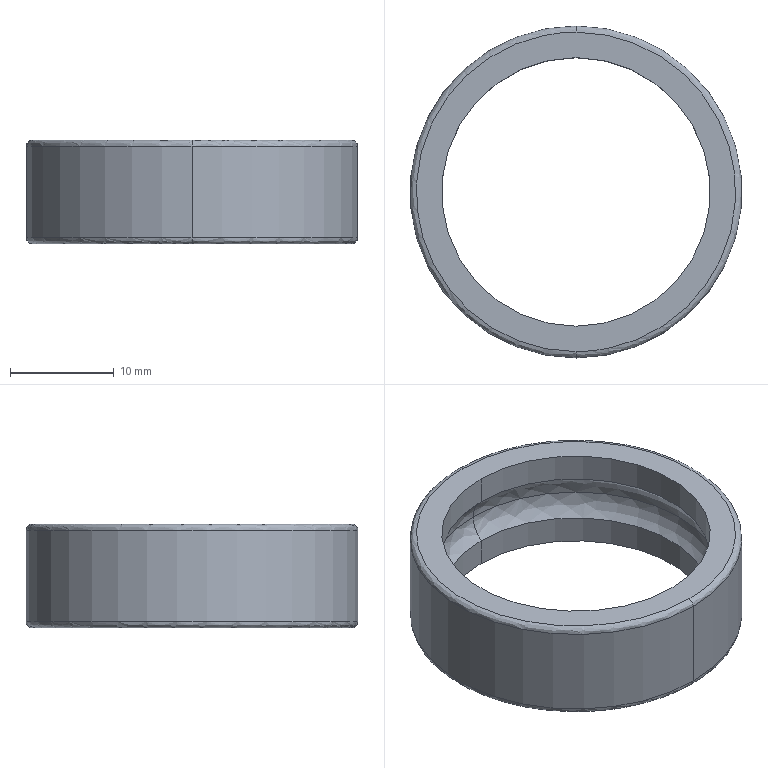Part | SolidWorks | features BaseBody 1 | 1 solid | 16 faces | box 32 x 32 x 10 mm | volume 2470 mm3 | spline 8 | cylinder 6 | plane 2 | commonest cylinder face diameters 25.9 x4 32 x2
STEP:
#1=CARTESIAN_POINT('',(0.,15.4,0.));
#2=VERTEX_POINT('',#1);
#3=CARTESIAN_POINT('',(0.,-15.4,0.));
#4=VERTEX_POINT('',#3);
#5=CARTESIAN_POINT('',(0.,15.4,0.));
#6=CARTESIAN_POINT('',(-30.8,15.4,0.));
#7=CARTESIAN_POINT('',(-30.8,-15.4,0.));
#8=CARTESIAN_POINT('',(0.,-15.4,0.));
#9=(BOUNDED_CURVE()B_SPLINE_CURVE(3,(#5,#6,#7,#8),.UNSPECIFIED.,.F.,.F.)B_SPLINE_CURVE_WITH_KNOTS((4,4),(0.25,0.75),.UNSPECIFIED.)CURVE()GEOMETRIC_REPRESENTATION_ITEM()RATIONAL_B_SPLINE_CURVE((1.,0.3333,0.3333,1.))REPRESENTATION_ITEM(''));
#10=EDGE_CURVE('',#2,#4,#9,.T.);
#11=ORIENTED_EDGE('',*,*,#10,.T.);
#12=CARTESIAN_POINT('',(0.,-16.,0.6));
#13=VERTEX_POINT('',#12);
#14=CARTESIAN_POINT('',(0.,-15.4,0.6));
#15=DIRECTION('',(-1.,0.,0.));
#16=DIRECTION('',(0.,-1.,0.));
#17=AXIS2_PLACEMENT_3D('',#14,#15,#16);
#18=CIRCLE('',#17,0.6);
#19=EDGE_CURVE('',#4,#13,#18,.T.);
#20=ORIENTED_EDGE('',*,*,#19,.T.);
#21=CARTESIAN_POINT('',(0.,16.,0.6));
#22=VERTEX_POINT('',#21);
#23=CARTESIAN_POINT('',(0.,0.,0.6));
#24=DIRECTION('',(0.,0.,1.));
#25=DIRECTION('',(0.,1.,0.));
#26=AXIS2_PLACEMENT_3D('',#23,#24,#25);
#27=CIRCLE('',#26,16.);
#28=EDGE_CURVE('',#22,#13,#27,.T.);
#29=ORIENTED_EDGE('',*,*,#28,.F.);
#30=CARTESIAN_POINT('',(0.,15.4,0.6));
#31=DIRECTION('',(1.,0.,0.));
#32=DIRECTION('',(0.,1.,0.));
#33=AXIS2_PLACEMENT_3D('',#30,#31,#32);
#34=CIRCLE('',#33,0.6);
#35=EDGE_CURVE('',#2,#22,#34,.T.);
#36=ORIENTED_EDGE('',*,*,#35,.F.);
#37=EDGE_LOOP('',(#11,#20,#29,#36));
#38=FACE_OUTER_BOUND('',#37,.T.);
#39=CARTESIAN_POINT('',(0.,-15.4,0.));
#40=CARTESIAN_POINT('',(-30.8,-15.4,0.));
#41=CARTESIAN_POINT('',(-30.8,15.4,0.));
#42=CARTESIAN_POINT('',(0.,15.4,0.));
#43=CARTESIAN_POINT('',(0.,-15.751,0.));
#44=CARTESIAN_POINT('',(-31.503,-15.751,0.));
#45=CARTESIAN_POINT('',(-31.503,15.751,0.));
#46=CARTESIAN_POINT('',(0.,15.751,0.));
#47=CARTESIAN_POINT('',(0.,-16.,0.2485));
#48=CARTESIAN_POINT('',(-32.,-16.,0.2485));
#49=CARTESIAN_POINT('',(-32.,16.,0.2485));
#50=CARTESIAN_POINT('',(0.,16.,0.2485));
#51=CARTESIAN_POINT('',(0.,-16.,0.6));
#52=CARTESIAN_POINT('',(-32.,-16.,0.6));
#53=CARTESIAN_POINT('',(-32.,16.,0.6));
#54=CARTESIAN_POINT('',(0.,16.,0.6));
#55=(BOUNDED_SURFACE()B_SPLINE_SURFACE(3,3,((#39,#40,#41,#42),(#43,#44,#45,#46),(#47,#48,#49,#50),(#51,#52,#53,#54)),.UNSPECIFIED.,.F.,.F.,.T.)B_SPLINE_SURFACE_WITH_KNOTS((4,4),(4,4),(0.,1.),(0.,1.),.UNSPECIFIED.)GEOMETRIC_REPRESENTATION_ITEM()RATIONAL_B_SPLINE_SURFACE(((1.,0.3333,0.3333,1.),(0.8047,0.2682,0.2682,0.8047),(0.8047,0.2682,0.2682,0.8047),(1.,0.3333,0.3333,1.)))REPRESENTATION_ITEM('')SURFACE());
#56=ADVANCED_FACE('',(#38),#55,.T.);
#57=CARTESIAN_POINT('',(0.,-16.,9.4));
#58=VERTEX_POINT('',#57);
#59=CARTESIAN_POINT('',(0.,16.,9.4));
#60=VERTEX_POINT('',#59);
#61=CARTESIAN_POINT('',(0.,0.,9.4));
#62=DIRECTION('',(0.,0.,-1.));
#63=DIRECTION('',(0.,1.,0.));
#64=AXIS2_PLACEMENT_3D('',#61,#62,#63);
#65=CIRCLE('',#64,16.);
#66=EDGE_CURVE('',#58,#60,#65,.T.);
#67=ORIENTED_EDGE('',*,*,#66,.F.);
#68=CARTESIAN_POINT('',(0.,-15.4,10.));
#69=VERTEX_POINT('',#68);
#70=CARTESIAN_POINT('',(0.,-15.4,9.4));
#71=DIRECTION('',(-1.,0.,0.));
#72=DIRECTION('',(0.,-1.,0.));
#73=AXIS2_PLACEMENT_3D('',#70,#71,#72);
#74=CIRCLE('',#73,0.6);
#75=EDGE_CURVE('',#58,#69,#74,.T.);
#76=ORIENTED_EDGE('',*,*,#75,.T.);
#77=CARTESIAN_POINT('',(0.,15.4,10.));
#78=VERTEX_POINT('',#77);
#79=CARTESIAN_POINT('',(0.,-15.4,10.));
#80=CARTESIAN_POINT('',(-30.8,-15.4,10.));
#81=CARTESIAN_POINT('',(-30.8,15.4,10.));
#82=CARTESIAN_POINT('',(0.,15.4,10.));
#83=(BOUNDED_CURVE()B_SPLINE_CURVE(3,(#79,#80,#81,#82),.UNSPECIFIED.,.F.,.F.)B_SPLINE_CURVE_WITH_KNOTS((4,4),(0.25,0.75),.UNSPECIFIED.)CURVE()GEOMETRIC_REPRESENTATION_ITEM()RATIONAL_B_SPLINE_CURVE((1.,0.3333,0.3333,1.))REPRESENTATION_ITEM(''));
#84=EDGE_CURVE('',#69,#78,#83,.T.);
#85=ORIENTED_EDGE('',*,*,#84,.T.);
#86=CARTESIAN_POINT('',(0.,15.4,9.4));
#87=DIRECTION('',(1.,0.,0.));
#88=DIRECTION('',(0.,1.,0.));
#89=AXIS2_PLACEMENT_3D('',#86,#87,#88);
#90=CIRCLE('',#89,0.6);
#91=EDGE_CURVE('',#60,#78,#90,.T.);
#92=ORIENTED_EDGE('',*,*,#91,.F.);
#93=EDGE_LOOP('',(#67,#76,#85,#92));
#94=FACE_OUTER_BOUND('',#93,.T.);
#95=CARTESIAN_POINT('',(0.,-16.,9.4));
#96=CARTESIAN_POINT('',(-32.,-16.,9.4));
#97=CARTESIAN_POINT('',(-32.,16.,9.4));
#98=CARTESIAN_POINT('',(0.,16.,9.4));
#99=CARTESIAN_POINT('',(0.,-16.,9.751));
#100=CARTESIAN_POINT('',(-32.,-16.,9.751));
#101=CARTESIAN_POINT('',(-32.,16.,9.751));
#102=CARTESIAN_POINT('',(0.,16.,9.751));
#103=CARTESIAN_POINT('',(0.,-15.751,10.));
#104=CARTESIAN_POINT('',(-31.503,-15.751,10.));
#105=CARTESIAN_POINT('',(-31.503,15.751,10.));
#106=CARTESIAN_POINT('',(0.,15.751,10.));
#107=CARTESIAN_POINT('',(0.,-15.4,10.));
#108=CARTESIAN_POINT('',(-30.8,-15.4,10.));
#109=CARTESIAN_POINT('',(-30.8,15.4,10.));
#110=CARTESIAN_POINT('',(0.,15.4,10.));
#111=(BOUNDED_SURFACE()B_SPLINE_SURFACE(3,3,((#95,#96,#97,#98),(#99,#100,#101,#102),(#103,#104,#105,#106),(#107,#108,#109,#110)),.UNSPECIFIED.,.F.,.F.,.T.)B_SPLINE_SURFACE_WITH_KNOTS((4,4),(4,4),(0.,1.),(0.,1.),.UNSPECIFIED.)GEOMETRIC_REPRESENTATION_ITEM()RATIONAL_B_SPLINE_SURFACE(((1.,0.3333,0.3333,1.),(0.8047,0.2682,0.2682,0.8047),(0.8047,0.2682,0.2682,0.8047),(1.,0.3333,0.3333,1.)))REPRESENTATION_ITEM('')SURFACE());
#112=ADVANCED_FACE('',(#94),#111,.T.);
#113=CARTESIAN_POINT('',(0.,12.95,2.699));
#114=VERTEX_POINT('',#113);
#115=CARTESIAN_POINT('',(0.,-12.95,2.699));
#116=VERTEX_POINT('',#115);
#117=CARTESIAN_POINT('',(0.,0.,2.699));
#118=DIRECTION('',(0.,0.,-1.));
#119=DIRECTION('',(0.,1.,0.));
#120=AXIS2_PLACEMENT_3D('',#117,#118,#119);
#121=CIRCLE('',#120,12.95);
#122=EDGE_CURVE('',#114,#116,#121,.T.);
#123=ORIENTED_EDGE('',*,*,#122,.T.);
#124=CARTESIAN_POINT('',(0.,-14.025,5.));
#125=VERTEX_POINT('',#124);
#126=CARTESIAN_POINT('',(0.,-11.025,5.));
#127=DIRECTION('',(-1.,0.,0.));
#128=DIRECTION('',(0.,-1.,0.));
#129=AXIS2_PLACEMENT_3D('',#126,#127,#128);
#130=CIRCLE('',#129,3.);
#131=EDGE_CURVE('',#116,#125,#130,.T.);
#132=ORIENTED_EDGE('',*,*,#131,.T.);
#133=CARTESIAN_POINT('',(0.,14.025,5.));
#134=VERTEX_POINT('',#133);
#135=CARTESIAN_POINT('',(0.,0.,5.));
#136=DIRECTION('',(0.,0.,-1.));
#137=DIRECTION('',(0.,1.,0.));
#138=AXIS2_PLACEMENT_3D('',#135,#136,#137);
#139=CIRCLE('',#138,14.025);
#140=EDGE_CURVE('',#134,#125,#139,.T.);
#141=ORIENTED_EDGE('',*,*,#140,.F.);
#142=CARTESIAN_POINT('',(0.,11.025,5.));
#143=DIRECTION('',(1.,0.,0.));
#144=DIRECTION('',(0.,1.,0.));
#145=AXIS2_PLACEMENT_3D('',#142,#143,#144);
#146=CIRCLE('',#145,3.);
#147=EDGE_CURVE('',#114,#134,#146,.T.);
#148=ORIENTED_EDGE('',*,*,#147,.F.);
#149=EDGE_LOOP('',(#123,#132,#141,#148));
#150=FACE_OUTER_BOUND('',#149,.T.);
#151=CARTESIAN_POINT('',(0.,12.95,2.699));
#152=CARTESIAN_POINT('',(25.9,12.95,2.699));
#153=CARTESIAN_POINT('',(25.9,-12.95,2.699));
#154=CARTESIAN_POINT('',(0.,-12.95,2.699));
#155=CARTESIAN_POINT('',(0.,13.643,3.279));
#156=CARTESIAN_POINT('',(27.285,13.643,3.279));
#157=CARTESIAN_POINT('',(27.285,-13.643,3.279));
#158=CARTESIAN_POINT('',(0.,-13.643,3.279));
#159=CARTESIAN_POINT('',(0.,14.025,4.097));
#160=CARTESIAN_POINT('',(28.05,14.025,4.097));
#161=CARTESIAN_POINT('',(28.05,-14.025,4.097));
#162=CARTESIAN_POINT('',(0.,-14.025,4.097));
#163=CARTESIAN_POINT('',(0.,14.025,5.));
#164=CARTESIAN_POINT('',(28.05,14.025,5.));
#165=CARTESIAN_POINT('',(28.05,-14.025,5.));
#166=CARTESIAN_POINT('',(0.,-14.025,5.));
#167=(BOUNDED_SURFACE()B_SPLINE_SURFACE(3,3,((#151,#152,#153,#154),(#155,#156,#157,#158),(#159,#160,#161,#162),(#163,#164,#165,#166)),.UNSPECIFIED.,.F.,.F.,.T.)B_SPLINE_SURFACE_WITH_KNOTS((4,4),(4,4),(0.,1.),(0.,1.),.UNSPECIFIED.)GEOMETRIC_REPRESENTATION_ITEM()RATIONAL_B_SPLINE_SURFACE(((1.,0.3333,0.3333,1.),(0.9373,0.3124,0.3124,0.9373),(0.9373,0.3124,0.3124,0.9373),(1.,0.3333,0.3333,1.)))REPRESENTATION_ITEM('')SURFACE());
#168=ADVANCED_FACE('',(#150),#167,.F.);
#169=ORIENTED_EDGE('',*,*,#140,.T.);
#170=CARTESIAN_POINT('',(0.,-12.95,7.301));
#171=VERTEX_POINT('',#170);
#172=CARTESIAN_POINT('',(0.,-11.025,5.));
#173=DIRECTION('',(-1.,0.,0.));
#174=DIRECTION('',(0.,-1.,0.));
#175=AXIS2_PLACEMENT_3D('',#172,#173,#174);
#176=CIRCLE('',#175,3.);
#177=EDGE_CURVE('',#125,#171,#176,.T.);
#178=ORIENTED_EDGE('',*,*,#177,.T.);
#179=CARTESIAN_POINT('',(0.,12.95,7.301));
#180=VERTEX_POINT('',#179);
#181=CARTESIAN_POINT('',(0.,0.,7.301));
#182=DIRECTION('',(0.,0.,1.));
#183=DIRECTION('',(0.,1.,0.));
#184=AXIS2_PLACEMENT_3D('',#181,#182,#183);
#185=CIRCLE('',#184,12.95);
#186=EDGE_CURVE('',#171,#180,#185,.T.);
#187=ORIENTED_EDGE('',*,*,#186,.T.);
#188=CARTESIAN_POINT('',(0.,11.025,5.));
#189=DIRECTION('',(1.,0.,0.));
#190=DIRECTION('',(0.,1.,0.));
#191=AXIS2_PLACEMENT_3D('',#188,#189,#190);
#192=CIRCLE('',#191,3.);
#193=EDGE_CURVE('',#134,#180,#192,.T.);
#194=ORIENTED_EDGE('',*,*,#193,.F.);
#195=EDGE_LOOP('',(#169,#178,#187,#194));
#196=FACE_OUTER_BOUND('',#195,.T.);
#197=CARTESIAN_POINT('',(0.,14.025,5.));
#198=CARTESIAN_POINT('',(28.05,14.025,5.));
#199=CARTESIAN_POINT('',(28.05,-14.025,5.));
#200=CARTESIAN_POINT('',(0.,-14.025,5.));
#201=CARTESIAN_POINT('',(0.,14.025,5.903));
#202=CARTESIAN_POINT('',(28.05,14.025,5.903));
#203=CARTESIAN_POINT('',(28.05,-14.025,5.903));
#204=CARTESIAN_POINT('',(0.,-14.025,5.903));
#205=CARTESIAN_POINT('',(0.,13.643,6.721));
#206=CARTESIAN_POINT('',(27.285,13.643,6.721));
#207=CARTESIAN_POINT('',(27.285,-13.643,6.721));
#208=CARTESIAN_POINT('',(0.,-13.643,6.721));
#209=CARTESIAN_POINT('',(0.,12.95,7.301));
#210=CARTESIAN_POINT('',(25.9,12.95,7.301));
#211=CARTESIAN_POINT('',(25.9,-12.95,7.301));
#212=CARTESIAN_POINT('',(0.,-12.95,7.301));
#213=(BOUNDED_SURFACE()B_SPLINE_SURFACE(3,3,((#197,#198,#199,#200),(#201,#202,#203,#204),(#205,#206,#207,#208),(#209,#210,#211,#212)),.UNSPECIFIED.,.F.,.F.,.F.)B_SPLINE_SURFACE_WITH_KNOTS((4,4),(4,4),(0.,1.),(0.,1.),.UNSPECIFIED.)GEOMETRIC_REPRESENTATION_ITEM()RATIONAL_B_SPLINE_SURFACE(((1.,0.3333,0.3333,1.),(0.9373,0.3124,0.3124,0.9373),(0.9373,0.3124,0.3124,0.9373),(1.,0.3333,0.3333,1.)))REPRESENTATION_ITEM('')SURFACE());
#214=ADVANCED_FACE('',(#196),#213,.F.);
#215=CARTESIAN_POINT('',(0.,0.,9.4));
#216=DIRECTION('',(0.,0.,-1.));
#217=DIRECTION('',(0.,1.,0.));
#218=AXIS2_PLACEMENT_3D('',#215,#216,#217);
#219=CIRCLE('',#218,16.);
#220=EDGE_CURVE('',#60,#58,#219,.T.);
#221=ORIENTED_EDGE('',*,*,#220,.T.);
#222=CARTESIAN_POINT('',(0.,-16.,0.));
#223=DIRECTION('',(0.,0.,-1.));
#224=VECTOR('',#223,1000.);
#225=LINE('',#222,#224);
#226=EDGE_CURVE('',#58,#13,#225,.T.);
#227=ORIENTED_EDGE('',*,*,#226,.T.);
#228=CARTESIAN_POINT('',(0.,0.,0.6));
#229=DIRECTION('',(0.,0.,1.));
#230=DIRECTION('',(0.,1.,0.));
#231=AXIS2_PLACEMENT_3D('',#228,#229,#230);
#232=CIRCLE('',#231,16.);
#233=EDGE_CURVE('',#13,#22,#232,.T.);
#234=ORIENTED_EDGE('',*,*,#233,.T.);
#235=CARTESIAN_POINT('',(0.,16.,0.));
#236=DIRECTION('',(0.,0.,-1.));
#237=VECTOR('',#236,1000.);
#238=LINE('',#235,#237);
#239=EDGE_CURVE('',#60,#22,#238,.T.);
#240=ORIENTED_EDGE('',*,*,#239,.F.);
#241=EDGE_LOOP('',(#221,#227,#234,#240));
#242=FACE_OUTER_BOUND('',#241,.T.);
#243=CARTESIAN_POINT('',(0.,0.,0.));
#244=DIRECTION('',(0.,0.,-1.));
#245=DIRECTION('',(0.,1.,0.));
#246=AXIS2_PLACEMENT_3D('',#243,#244,#245);
#247=CYLINDRICAL_SURFACE('',#246,16.);
#248=ADVANCED_FACE('',(#242),#247,.T.);
#249=CARTESIAN_POINT('',(0.,0.,2.699));
#250=DIRECTION('',(0.,0.,-1.));
#251=DIRECTION('',(0.,1.,0.));
#252=AXIS2_PLACEMENT_3D('',#249,#250,#251);
#253=CIRCLE('',#252,12.95);
#254=EDGE_CURVE('',#116,#114,#253,.T.);
#255=ORIENTED_EDGE('',*,*,#254,.F.);
#256=CARTESIAN_POINT('',(0.,-12.95,0.));
#257=VERTEX_POINT('',#256);
#258=CARTESIAN_POINT('',(0.,-12.95,0.));
#259=DIRECTION('',(0.,0.,-1.));
#260=VECTOR('',#259,1000.);
#261=LINE('',#258,#260);
#262=EDGE_CURVE('',#116,#257,#261,.T.);
#263=ORIENTED_EDGE('',*,*,#262,.T.);
#264=CARTESIAN_POINT('',(0.,12.95,0.));
#265=VERTEX_POINT('',#264);
#266=CARTESIAN_POINT('',(0.,0.,0.));
#267=DIRECTION('',(0.,0.,1.));
#268=DIRECTION('',(0.,1.,0.));
#269=AXIS2_PLACEMENT_3D('',#266,#267,#268);
#270=CIRCLE('',#269,12.95);
#271=EDGE_CURVE('',#265,#257,#270,.T.);
#272=ORIENTED_EDGE('',*,*,#271,.F.);
#273=CARTESIAN_POINT('',(0.,12.95,0.));
#274=DIRECTION('',(0.,0.,-1.));
#275=VECTOR('',#274,1000.);
#276=LINE('',#273,#275);
#277=EDGE_CURVE('',#114,#265,#276,.T.);
#278=ORIENTED_EDGE('',*,*,#277,.F.);
#279=EDGE_LOOP('',(#255,#263,#272,#278));
#280=FACE_OUTER_BOUND('',#279,.T.);
#281=CARTESIAN_POINT('',(0.,0.,0.));
#282=DIRECTION('',(0.,0.,-1.));
#283=DIRECTION('',(0.,1.,0.));
#284=AXIS2_PLACEMENT_3D('',#281,#282,#283);
#285=CYLINDRICAL_SURFACE('',#284,12.95);
#286=ADVANCED_FACE('',(#280),#285,.F.);
#287=CARTESIAN_POINT('',(0.,-12.95,10.));
#288=VERTEX_POINT('',#287);
#289=CARTESIAN_POINT('',(0.,12.95,10.));
#290=VERTEX_POINT('',#289);
#291=CARTESIAN_POINT('',(0.,0.,10.));
#292=DIRECTION('',(0.,0.,-1.));
#293=DIRECTION('',(0.,1.,0.));
#294=AXIS2_PLACEMENT_3D('',#291,#292,#293);
#295=CIRCLE('',#294,12.95);
#296=EDGE_CURVE('',#288,#290,#295,.T.);
#297=ORIENTED_EDGE('',*,*,#296,.F.);
#298=CARTESIAN_POINT('',(0.,-12.95,0.));
#299=DIRECTION('',(0.,0.,-1.));
#300=VECTOR('',#299,1000.);
#301=LINE('',#298,#300);
#302=EDGE_CURVE('',#288,#171,#301,.T.);
#303=ORIENTED_EDGE('',*,*,#302,.T.);
#304=CARTESIAN_POINT('',(0.,0.,7.301));
#305=DIRECTION('',(0.,0.,1.));
#306=DIRECTION('',(0.,1.,0.));
#307=AXIS2_PLACEMENT_3D('',#304,#305,#306);
#308=CIRCLE('',#307,12.95);
#309=EDGE_CURVE('',#180,#171,#308,.T.);
#310=ORIENTED_EDGE('',*,*,#309,.F.);
#311=CARTESIAN_POINT('',(0.,12.95,0.));
#312=DIRECTION('',(0.,0.,-1.));
#313=VECTOR('',#312,1000.);
#314=LINE('',#311,#313);
#315=EDGE_CURVE('',#290,#180,#314,.T.);
#316=ORIENTED_EDGE('',*,*,#315,.F.);
#317=EDGE_LOOP('',(#297,#303,#310,#316));
#318=FACE_OUTER_BOUND('',#317,.T.);
#319=CARTESIAN_POINT('',(0.,0.,0.));
#320=DIRECTION('',(0.,0.,-1.));
#321=DIRECTION('',(0.,1.,0.));
#322=AXIS2_PLACEMENT_3D('',#319,#320,#321);
#323=CYLINDRICAL_SURFACE('',#322,12.95);
#324=ADVANCED_FACE('',(#318),#323,.F.);
#325=ORIENTED_EDGE('',*,*,#177,.F.);
#326=CARTESIAN_POINT('',(0.,0.,5.));
#327=DIRECTION('',(0.,0.,-1.));
#328=DIRECTION('',(0.,1.,0.));
#329=AXIS2_PLACEMENT_3D('',#326,#327,#328);
#330=CIRCLE('',#329,14.025);
#331=EDGE_CURVE('',#125,#134,#330,.T.);
#332=ORIENTED_EDGE('',*,*,#331,.T.);
#333=ORIENTED_EDGE('',*,*,#193,.T.);
#334=ORIENTED_EDGE('',*,*,#309,.T.);
#335=EDGE_LOOP('',(#325,#332,#333,#334));
#336=FACE_OUTER_BOUND('',#335,.T.);
#337=CARTESIAN_POINT('',(0.,-14.025,5.));
#338=CARTESIAN_POINT('',(-28.05,-14.025,5.));
#339=CARTESIAN_POINT('',(-28.05,14.025,5.));
#340=CARTESIAN_POINT('',(0.,14.025,5.));
#341=CARTESIAN_POINT('',(0.,-14.025,5.903));
#342=CARTESIAN_POINT('',(-28.05,-14.025,5.903));
#343=CARTESIAN_POINT('',(-28.05,14.025,5.903));
#344=CARTESIAN_POINT('',(0.,14.025,5.903));
#345=CARTESIAN_POINT('',(0.,-13.643,6.721));
#346=CARTESIAN_POINT('',(-27.285,-13.643,6.721));
#347=CARTESIAN_POINT('',(-27.285,13.643,6.721));
#348=CARTESIAN_POINT('',(0.,13.643,6.721));
#349=CARTESIAN_POINT('',(0.,-12.95,7.301));
#350=CARTESIAN_POINT('',(-25.9,-12.95,7.301));
#351=CARTESIAN_POINT('',(-25.9,12.95,7.301));
#352=CARTESIAN_POINT('',(0.,12.95,7.301));
#353=(BOUNDED_SURFACE()B_SPLINE_SURFACE(3,3,((#337,#338,#339,#340),(#341,#342,#343,#344),(#345,#346,#347,#348),(#349,#350,#351,#352)),.UNSPECIFIED.,.F.,.F.,.T.)B_SPLINE_SURFACE_WITH_KNOTS((4,4),(4,4),(0.,1.),(0.,1.),.UNSPECIFIED.)GEOMETRIC_REPRESENTATION_ITEM()RATIONAL_B_SPLINE_SURFACE(((1.,0.3333,0.3333,1.),(0.9373,0.3124,0.3124,0.9373),(0.9373,0.3124,0.3124,0.9373),(1.,0.3333,0.3333,1.)))REPRESENTATION_ITEM('')SURFACE());
#354=ADVANCED_FACE('',(#336),#353,.F.);
#355=ORIENTED_EDGE('',*,*,#226,.F.);
#356=ORIENTED_EDGE('',*,*,#66,.T.);
#357=ORIENTED_EDGE('',*,*,#239,.T.);
#358=ORIENTED_EDGE('',*,*,#28,.T.);
#359=EDGE_LOOP('',(#355,#356,#357,#358));
#360=FACE_OUTER_BOUND('',#359,.T.);
#361=CARTESIAN_POINT('',(0.,0.,0.));
#362=DIRECTION('',(0.,0.,-1.));
#363=DIRECTION('',(0.,1.,0.));
#364=AXIS2_PLACEMENT_3D('',#361,#362,#363);
#365=CYLINDRICAL_SURFACE('',#364,16.);
#366=ADVANCED_FACE('',(#360),#365,.T.);
#367=ORIENTED_EDGE('',*,*,#19,.F.);
#368=CARTESIAN_POINT('',(0.,-15.4,0.));
#369=CARTESIAN_POINT('',(30.8,-15.4,0.));
#370=CARTESIAN_POINT('',(30.8,15.4,0.));
#371=CARTESIAN_POINT('',(0.,15.4,0.));
#372=(BOUNDED_CURVE()B_SPLINE_CURVE(3,(#368,#369,#370,#371),.UNSPECIFIED.,.F.,.F.)B_SPLINE_CURVE_WITH_KNOTS((4,4),(0.75,1.25),.UNSPECIFIED.)CURVE()GEOMETRIC_REPRESENTATION_ITEM()RATIONAL_B_SPLINE_CURVE((1.,0.3333,0.3333,1.))REPRESENTATION_ITEM(''));
#373=EDGE_CURVE('',#4,#2,#372,.T.);
#374=ORIENTED_EDGE('',*,*,#373,.T.);
#375=ORIENTED_EDGE('',*,*,#35,.T.);
#376=ORIENTED_EDGE('',*,*,#233,.F.);
#377=EDGE_LOOP('',(#367,#374,#375,#376));
#378=FACE_OUTER_BOUND('',#377,.T.);
#379=CARTESIAN_POINT('',(0.,15.4,0.));
#380=CARTESIAN_POINT('',(30.8,15.4,0.));
#381=CARTESIAN_POINT('',(30.8,-15.4,0.));
#382=CARTESIAN_POINT('',(0.,-15.4,0.));
#383=CARTESIAN_POINT('',(0.,15.751,0.));
#384=CARTESIAN_POINT('',(31.503,15.751,0.));
#385=CARTESIAN_POINT('',(31.503,-15.751,0.));
#386=CARTESIAN_POINT('',(0.,-15.751,0.));
#387=CARTESIAN_POINT('',(0.,16.,0.2485));
#388=CARTESIAN_POINT('',(32.,16.,0.2485));
#389=CARTESIAN_POINT('',(32.,-16.,0.2485));
#390=CARTESIAN_POINT('',(0.,-16.,0.2485));
#391=CARTESIAN_POINT('',(0.,16.,0.6));
#392=CARTESIAN_POINT('',(32.,16.,0.6));
#393=CARTESIAN_POINT('',(32.,-16.,0.6));
#394=CARTESIAN_POINT('',(0.,-16.,0.6));
#395=(BOUNDED_SURFACE()B_SPLINE_SURFACE(3,3,((#379,#380,#381,#382),(#383,#384,#385,#386),(#387,#388,#389,#390),(#391,#392,#393,#394)),.UNSPECIFIED.,.F.,.F.,.T.)B_SPLINE_SURFACE_WITH_KNOTS((4,4),(4,4),(0.,1.),(0.,1.),.UNSPECIFIED.)GEOMETRIC_REPRESENTATION_ITEM()RATIONAL_B_SPLINE_SURFACE(((1.,0.3333,0.3333,1.),(0.8047,0.2682,0.2682,0.8047),(0.8047,0.2682,0.2682,0.8047),(1.,0.3333,0.3333,1.)))REPRESENTATION_ITEM('')SURFACE());
#396=ADVANCED_FACE('',(#378),#395,.T.);
#397=ORIENTED_EDGE('',*,*,#75,.F.);
#398=ORIENTED_EDGE('',*,*,#220,.F.);
#399=ORIENTED_EDGE('',*,*,#91,.T.);
#400=CARTESIAN_POINT('',(0.,15.4,10.));
#401=CARTESIAN_POINT('',(30.8,15.4,10.));
#402=CARTESIAN_POINT('',(30.8,-15.4,10.));
#403=CARTESIAN_POINT('',(0.,-15.4,10.));
#404=(BOUNDED_CURVE()B_SPLINE_CURVE(3,(#400,#401,#402,#403),.UNSPECIFIED.,.F.,.F.)B_SPLINE_CURVE_WITH_KNOTS((4,4),(0.75,1.25),.UNSPECIFIED.)CURVE()GEOMETRIC_REPRESENTATION_ITEM()RATIONAL_B_SPLINE_CURVE((1.,0.3333,0.3333,1.))REPRESENTATION_ITEM(''));
#405=EDGE_CURVE('',#78,#69,#404,.T.);
#406=ORIENTED_EDGE('',*,*,#405,.T.);
#407=EDGE_LOOP('',(#397,#398,#399,#406));
#408=FACE_OUTER_BOUND('',#407,.T.);
#409=CARTESIAN_POINT('',(0.,16.,9.4));
#410=CARTESIAN_POINT('',(32.,16.,9.4));
#411=CARTESIAN_POINT('',(32.,-16.,9.4));
#412=CARTESIAN_POINT('',(0.,-16.,9.4));
#413=CARTESIAN_POINT('',(0.,16.,9.751));
#414=CARTESIAN_POINT('',(32.,16.,9.751));
#415=CARTESIAN_POINT('',(32.,-16.,9.751));
#416=CARTESIAN_POINT('',(0.,-16.,9.751));
#417=CARTESIAN_POINT('',(0.,15.751,10.));
#418=CARTESIAN_POINT('',(31.503,15.751,10.));
#419=CARTESIAN_POINT('',(31.503,-15.751,10.));
#420=CARTESIAN_POINT('',(0.,-15.751,10.));
#421=CARTESIAN_POINT('',(0.,15.4,10.));
#422=CARTESIAN_POINT('',(30.8,15.4,10.));
#423=CARTESIAN_POINT('',(30.8,-15.4,10.));
#424=CARTESIAN_POINT('',(0.,-15.4,10.));
#425=(BOUNDED_SURFACE()B_SPLINE_SURFACE(3,3,((#409,#410,#411,#412),(#413,#414,#415,#416),(#417,#418,#419,#420),(#421,#422,#423,#424)),.UNSPECIFIED.,.F.,.F.,.T.)B_SPLINE_SURFACE_WITH_KNOTS((4,4),(4,4),(0.,1.),(0.,1.),.UNSPECIFIED.)GEOMETRIC_REPRESENTATION_ITEM()RATIONAL_B_SPLINE_SURFACE(((1.,0.3333,0.3333,1.),(0.8047,0.2682,0.2682,0.8047),(0.8047,0.2682,0.2682,0.8047),(1.,0.3333,0.3333,1.)))REPRESENTATION_ITEM('')SURFACE());
#426=ADVANCED_FACE('',(#408),#425,.T.);
#427=ORIENTED_EDGE('',*,*,#271,.T.);
#428=CARTESIAN_POINT('',(0.,0.,0.));
#429=DIRECTION('',(0.,0.,1.));
#430=DIRECTION('',(0.,1.,0.));
#431=AXIS2_PLACEMENT_3D('',#428,#429,#430);
#432=CIRCLE('',#431,12.95);
#433=EDGE_CURVE('',#257,#265,#432,.T.);
#434=ORIENTED_EDGE('',*,*,#433,.T.);
#435=EDGE_LOOP('',(#427,#434));
#436=FACE_BOUND('',#435,.T.);
#437=ORIENTED_EDGE('',*,*,#10,.F.);
#438=ORIENTED_EDGE('',*,*,#373,.F.);
#439=EDGE_LOOP('',(#437,#438));
#440=FACE_OUTER_BOUND('',#439,.T.);
#441=CARTESIAN_POINT('',(12.95,0.,0.));
#442=DIRECTION('',(0.,0.,-1.));
#443=DIRECTION('',(0.,1.,0.));
#444=AXIS2_PLACEMENT_3D('',#441,#442,#443);
#445=PLANE('',#444);
#446=ADVANCED_FACE('',(#436,#440),#445,.T.);
#447=ORIENTED_EDGE('',*,*,#405,.F.);
#448=ORIENTED_EDGE('',*,*,#84,.F.);
#449=EDGE_LOOP('',(#447,#448));
#450=FACE_OUTER_BOUND('',#449,.T.);
#451=CARTESIAN_POINT('',(0.,0.,10.));
#452=DIRECTION('',(0.,0.,-1.));
#453=DIRECTION('',(0.,1.,0.));
#454=AXIS2_PLACEMENT_3D('',#451,#452,#453);
#455=CIRCLE('',#454,12.95);
#456=EDGE_CURVE('',#290,#288,#455,.T.);
#457=ORIENTED_EDGE('',*,*,#456,.T.);
#458=ORIENTED_EDGE('',*,*,#296,.T.);
#459=EDGE_LOOP('',(#457,#458));
#460=FACE_BOUND('',#459,.T.);
#461=CARTESIAN_POINT('',(15.4,0.,10.));
#462=DIRECTION('',(0.,0.,1.));
#463=DIRECTION('',(0.,-1.,0.));
#464=AXIS2_PLACEMENT_3D('',#461,#462,#463);
#465=PLANE('',#464);
#466=ADVANCED_FACE('',(#450,#460),#465,.T.);
#467=ORIENTED_EDGE('',*,*,#262,.F.);
#468=ORIENTED_EDGE('',*,*,#122,.F.);
#469=ORIENTED_EDGE('',*,*,#277,.T.);
#470=ORIENTED_EDGE('',*,*,#433,.F.);
#471=EDGE_LOOP('',(#467,#468,#469,#470));
#472=FACE_OUTER_BOUND('',#471,.T.);
#473=CARTESIAN_POINT('',(0.,0.,0.));
#474=DIRECTION('',(0.,0.,-1.));
#475=DIRECTION('',(0.,1.,0.));
#476=AXIS2_PLACEMENT_3D('',#473,#474,#475);
#477=CYLINDRICAL_SURFACE('',#476,12.95);
#478=ADVANCED_FACE('',(#472),#477,.F.);
#479=ORIENTED_EDGE('',*,*,#302,.F.);
#480=ORIENTED_EDGE('',*,*,#456,.F.);
#481=ORIENTED_EDGE('',*,*,#315,.T.);
#482=ORIENTED_EDGE('',*,*,#186,.F.);
#483=EDGE_LOOP('',(#479,#480,#481,#482));
#484=FACE_OUTER_BOUND('',#483,.T.);
#485=CARTESIAN_POINT('',(0.,0.,0.));
#486=DIRECTION('',(0.,0.,-1.));
#487=DIRECTION('',(0.,1.,0.));
#488=AXIS2_PLACEMENT_3D('',#485,#486,#487);
#489=CYLINDRICAL_SURFACE('',#488,12.95);
#490=ADVANCED_FACE('',(#484),#489,.F.);
#491=ORIENTED_EDGE('',*,*,#131,.F.);
#492=ORIENTED_EDGE('',*,*,#254,.T.);
#493=ORIENTED_EDGE('',*,*,#147,.T.);
#494=ORIENTED_EDGE('',*,*,#331,.F.);
#495=EDGE_LOOP('',(#491,#492,#493,#494));
#496=FACE_OUTER_BOUND('',#495,.T.);
#497=CARTESIAN_POINT('',(0.,-12.95,2.699));
#498=CARTESIAN_POINT('',(-25.9,-12.95,2.699));
#499=CARTESIAN_POINT('',(-25.9,12.95,2.699));
#500=CARTESIAN_POINT('',(0.,12.95,2.699));
#501=CARTESIAN_POINT('',(0.,-13.643,3.279));
#502=CARTESIAN_POINT('',(-27.285,-13.643,3.279));
#503=CARTESIAN_POINT('',(-27.285,13.643,3.279));
#504=CARTESIAN_POINT('',(0.,13.643,3.279));
#505=CARTESIAN_POINT('',(0.,-14.025,4.097));
#506=CARTESIAN_POINT('',(-28.05,-14.025,4.097));
#507=CARTESIAN_POINT('',(-28.05,14.025,4.097));
#508=CARTESIAN_POINT('',(0.,14.025,4.097));
#509=CARTESIAN_POINT('',(0.,-14.025,5.));
#510=CARTESIAN_POINT('',(-28.05,-14.025,5.));
#511=CARTESIAN_POINT('',(-28.05,14.025,5.));
#512=CARTESIAN_POINT('',(0.,14.025,5.));
#513=(BOUNDED_SURFACE()B_SPLINE_SURFACE(3,3,((#497,#498,#499,#500),(#501,#502,#503,#504),(#505,#506,#507,#508),(#509,#510,#511,#512)),.UNSPECIFIED.,.F.,.F.,.F.)B_SPLINE_SURFACE_WITH_KNOTS((4,4),(4,4),(0.,1.),(0.,1.),.UNSPECIFIED.)GEOMETRIC_REPRESENTATION_ITEM()RATIONAL_B_SPLINE_SURFACE(((1.,0.3333,0.3333,1.),(0.9373,0.3124,0.3124,0.9373),(0.9373,0.3124,0.3124,0.9373),(1.,0.3333,0.3333,1.)))REPRESENTATION_ITEM('')SURFACE());
#514=ADVANCED_FACE('',(#496),#513,.F.);
#515=CLOSED_SHELL('',(#56,#112,#168,#214,#248,#286,#324,#354,#366,#396,#426,#446,#466,#478,#490,#514));
#516=MANIFOLD_SOLID_BREP('',#515);
#517=CARTESIAN_POINT('',(0.,0.,0.));
#518=DIRECTION('',(0.,0.,1.));
#519=DIRECTION('',(1.,0.,0.));
#520=AXIS2_PLACEMENT_3D('',#517,#518,#519);
#521=(LENGTH_UNIT()NAMED_UNIT(*)SI_UNIT(.MILLI.,.METRE.));
#522=UNCERTAINTY_MEASURE_WITH_UNIT(LENGTH_MEASURE(0.00001),#521,'','');
#523=(NAMED_UNIT(*)PLANE_ANGLE_UNIT()SI_UNIT($,.RADIAN.));
#524=(NAMED_UNIT(*)SI_UNIT($,.STERADIAN.)SOLID_ANGLE_UNIT());
#525=(GEOMETRIC_REPRESENTATION_CONTEXT(3)GLOBAL_UNCERTAINTY_ASSIGNED_CONTEXT((#522))GLOBAL_UNIT_ASSIGNED_CONTEXT((#521,#523,#524))REPRESENTATION_CONTEXT('',''));
#526=ADVANCED_BREP_SHAPE_REPRESENTATION('',(#516,#520),#525);